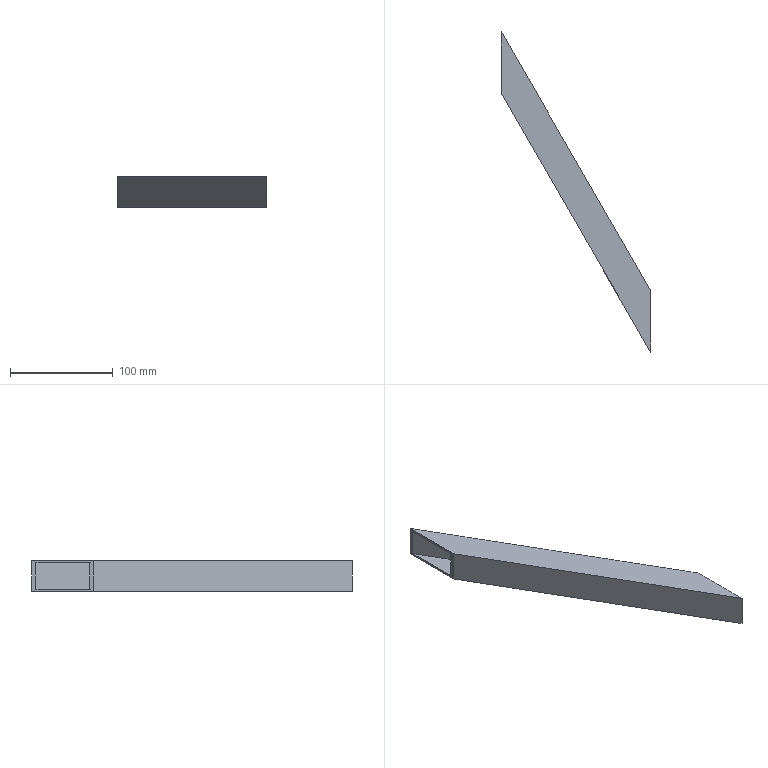Part | NX | features solid 2 | 1 solid | 10 faces | box 145 x 311.147 x 30 mm | volume 64960 mm3 | plane 10
STEP:
#1=CARTESIAN_POINT('',(-115.,495.,-45.));
#2=VERTEX_POINT('',#1);
#3=CARTESIAN_POINT('',(-115.,495.,-75.));
#4=VERTEX_POINT('',#3);
#5=CARTESIAN_POINT('',(-115.,495.,-75.));
#6=DIRECTION('',(0.,0.,-1.));
#7=VECTOR('',#6,1000.);
#8=LINE('',#5,#7);
#9=EDGE_CURVE('',#2,#4,#8,.T.);
#10=ORIENTED_EDGE('',*,*,#9,.F.);
#11=CARTESIAN_POINT('',(30.,243.853,-45.));
#12=VERTEX_POINT('',#11);
#13=CARTESIAN_POINT('',(-89.019,450.,-45.));
#14=DIRECTION('',(0.5,-0.866,0.));
#15=VECTOR('',#14,1000.);
#16=LINE('',#13,#15);
#17=EDGE_CURVE('',#2,#12,#16,.T.);
#18=ORIENTED_EDGE('',*,*,#17,.T.);
#19=CARTESIAN_POINT('',(30.,243.853,-75.));
#20=VERTEX_POINT('',#19);
#21=CARTESIAN_POINT('',(30.,243.853,-75.));
#22=DIRECTION('',(0.,0.,1.));
#23=VECTOR('',#22,1000.);
#24=LINE('',#21,#23);
#25=EDGE_CURVE('',#20,#12,#24,.T.);
#26=ORIENTED_EDGE('',*,*,#25,.F.);
#27=CARTESIAN_POINT('',(-89.019,450.,-75.));
#28=DIRECTION('',(0.5,-0.866,0.));
#29=VECTOR('',#28,1000.);
#30=LINE('',#27,#29);
#31=EDGE_CURVE('',#4,#20,#30,.T.);
#32=ORIENTED_EDGE('',*,*,#31,.F.);
#33=EDGE_LOOP('',(#10,#18,#26,#32));
#34=FACE_BOUND('',#33,.T.);
#35=CARTESIAN_POINT('',(-89.019,450.,-75.));
#36=DIRECTION('',(0.866,0.5,0.));
#37=DIRECTION('',(0.,0.,1.));
#38=AXIS2_PLACEMENT_3D('',#35,#36,#37);
#39=PLANE('',#38);
#40=ADVANCED_FACE('',(#34),#39,.T.);
#41=CARTESIAN_POINT('',(-115.,435.,-45.));
#42=VERTEX_POINT('',#41);
#43=CARTESIAN_POINT('',(30.,183.853,-45.));
#44=VERTEX_POINT('',#43);
#45=CARTESIAN_POINT('',(-115.,435.,-45.));
#46=DIRECTION('',(0.5,-0.866,0.));
#47=VECTOR('',#46,1000.);
#48=LINE('',#45,#47);
#49=EDGE_CURVE('',#42,#44,#48,.T.);
#50=ORIENTED_EDGE('',*,*,#49,.F.);
#51=CARTESIAN_POINT('',(-115.,435.,-75.));
#52=VERTEX_POINT('',#51);
#53=CARTESIAN_POINT('',(-115.,435.,-75.));
#54=DIRECTION('',(0.,0.,-1.));
#55=VECTOR('',#54,1000.);
#56=LINE('',#53,#55);
#57=EDGE_CURVE('',#42,#52,#56,.T.);
#58=ORIENTED_EDGE('',*,*,#57,.T.);
#59=CARTESIAN_POINT('',(30.,183.853,-75.));
#60=VERTEX_POINT('',#59);
#61=CARTESIAN_POINT('',(-115.,435.,-75.));
#62=DIRECTION('',(0.5,-0.866,0.));
#63=VECTOR('',#62,1000.);
#64=LINE('',#61,#63);
#65=EDGE_CURVE('',#52,#60,#64,.T.);
#66=ORIENTED_EDGE('',*,*,#65,.T.);
#67=CARTESIAN_POINT('',(30.,183.853,-75.));
#68=DIRECTION('',(0.,0.,1.));
#69=VECTOR('',#68,1000.);
#70=LINE('',#67,#69);
#71=EDGE_CURVE('',#60,#44,#70,.T.);
#72=ORIENTED_EDGE('',*,*,#71,.T.);
#73=EDGE_LOOP('',(#50,#58,#66,#72));
#74=FACE_BOUND('',#73,.T.);
#75=CARTESIAN_POINT('',(-115.,435.,-75.));
#76=DIRECTION('',(0.866,0.5,0.));
#77=DIRECTION('',(0.,0.,1.));
#78=AXIS2_PLACEMENT_3D('',#75,#76,#77);
#79=PLANE('',#78);
#80=ADVANCED_FACE('',(#74),#79,.F.);
#81=ORIENTED_EDGE('',*,*,#65,.F.);
#82=CARTESIAN_POINT('',(-115.,450.,-75.));
#83=DIRECTION('',(0.,1.,0.));
#84=VECTOR('',#83,1000.);
#85=LINE('',#82,#84);
#86=EDGE_CURVE('',#52,#4,#85,.T.);
#87=ORIENTED_EDGE('',*,*,#86,.T.);
#88=ORIENTED_EDGE('',*,*,#31,.T.);
#89=CARTESIAN_POINT('',(30.,450.,-75.));
#90=DIRECTION('',(0.,-1.,0.));
#91=VECTOR('',#90,1000.);
#92=LINE('',#89,#91);
#93=EDGE_CURVE('',#20,#60,#92,.T.);
#94=ORIENTED_EDGE('',*,*,#93,.T.);
#95=EDGE_LOOP('',(#81,#87,#88,#94));
#96=FACE_BOUND('',#95,.T.);
#97=CARTESIAN_POINT('',(-89.019,450.,-75.));
#98=DIRECTION('',(0.,0.,1.));
#99=DIRECTION('',(0.5,-0.866,0.));
#100=AXIS2_PLACEMENT_3D('',#97,#98,#99);
#101=PLANE('',#100);
#102=ADVANCED_FACE('',(#96),#101,.F.);
#103=ORIENTED_EDGE('',*,*,#17,.F.);
#104=CARTESIAN_POINT('',(-115.,450.,-45.));
#105=DIRECTION('',(0.,1.,0.));
#106=VECTOR('',#105,1000.);
#107=LINE('',#104,#106);
#108=EDGE_CURVE('',#2,#42,#107,.F.);
#109=ORIENTED_EDGE('',*,*,#108,.T.);
#110=ORIENTED_EDGE('',*,*,#49,.T.);
#111=CARTESIAN_POINT('',(30.,115.,-45.));
#112=DIRECTION('',(0.,1.,0.));
#113=VECTOR('',#112,1000.);
#114=LINE('',#111,#113);
#115=EDGE_CURVE('',#12,#44,#114,.F.);
#116=ORIENTED_EDGE('',*,*,#115,.F.);
#117=EDGE_LOOP('',(#103,#109,#110,#116));
#118=FACE_BOUND('',#117,.T.);
#119=CARTESIAN_POINT('',(-89.019,450.,-45.));
#120=DIRECTION('',(0.,0.,1.));
#121=DIRECTION('',(0.5,-0.866,0.));
#122=AXIS2_PLACEMENT_3D('',#119,#120,#121);
#123=PLANE('',#122);
#124=ADVANCED_FACE('',(#118),#123,.T.);
#125=ORIENTED_EDGE('',*,*,#115,.T.);
#126=ORIENTED_EDGE('',*,*,#71,.F.);
#127=ORIENTED_EDGE('',*,*,#93,.F.);
#128=ORIENTED_EDGE('',*,*,#25,.T.);
#129=EDGE_LOOP('',(#125,#126,#127,#128));
#130=FACE_BOUND('',#129,.T.);
#131=CARTESIAN_POINT('',(30.,239.853,-47.));
#132=VERTEX_POINT('',#131);
#133=CARTESIAN_POINT('',(30.,187.853,-47.));
#134=VERTEX_POINT('',#133);
#135=CARTESIAN_POINT('',(30.,115.,-47.));
#136=DIRECTION('',(0.,1.,0.));
#137=VECTOR('',#136,1000.);
#138=LINE('',#135,#137);
#139=EDGE_CURVE('',#132,#134,#138,.F.);
#140=ORIENTED_EDGE('',*,*,#139,.F.);
#141=CARTESIAN_POINT('',(30.,239.853,-73.));
#142=VERTEX_POINT('',#141);
#143=CARTESIAN_POINT('',(30.,239.853,-75.));
#144=DIRECTION('',(0.,0.,1.));
#145=VECTOR('',#144,1000.);
#146=LINE('',#143,#145);
#147=EDGE_CURVE('',#142,#132,#146,.T.);
#148=ORIENTED_EDGE('',*,*,#147,.F.);
#149=CARTESIAN_POINT('',(30.,187.853,-73.));
#150=VERTEX_POINT('',#149);
#151=CARTESIAN_POINT('',(30.,450.,-73.));
#152=DIRECTION('',(0.,-1.,0.));
#153=VECTOR('',#152,1000.);
#154=LINE('',#151,#153);
#155=EDGE_CURVE('',#142,#150,#154,.T.);
#156=ORIENTED_EDGE('',*,*,#155,.T.);
#157=CARTESIAN_POINT('',(30.,187.853,-75.));
#158=DIRECTION('',(0.,0.,1.));
#159=VECTOR('',#158,1000.);
#160=LINE('',#157,#159);
#161=EDGE_CURVE('',#150,#134,#160,.T.);
#162=ORIENTED_EDGE('',*,*,#161,.T.);
#163=EDGE_LOOP('',(#140,#148,#156,#162));
#164=FACE_BOUND('',#163,.T.);
#165=CARTESIAN_POINT('',(30.,115.,-45.));
#166=DIRECTION('',(-1.,0.,0.));
#167=DIRECTION('',(0.,-1.,0.));
#168=AXIS2_PLACEMENT_3D('',#165,#166,#167);
#169=PLANE('',#168);
#170=ADVANCED_FACE('',(#130,#164),#169,.F.);
#171=CARTESIAN_POINT('',(-115.,491.,-47.));
#172=VERTEX_POINT('',#171);
#173=CARTESIAN_POINT('',(-90.751,449.,-47.));
#174=DIRECTION('',(-0.5,0.866,0.));
#175=VECTOR('',#174,1000.);
#176=LINE('',#173,#175);
#177=EDGE_CURVE('',#172,#132,#176,.F.);
#178=ORIENTED_EDGE('',*,*,#177,.F.);
#179=CARTESIAN_POINT('',(-115.,491.,-73.));
#180=VERTEX_POINT('',#179);
#181=CARTESIAN_POINT('',(-115.,491.,-75.));
#182=DIRECTION('',(0.,0.,-1.));
#183=VECTOR('',#182,1000.);
#184=LINE('',#181,#183);
#185=EDGE_CURVE('',#172,#180,#184,.T.);
#186=ORIENTED_EDGE('',*,*,#185,.T.);
#187=CARTESIAN_POINT('',(-90.751,449.,-73.));
#188=DIRECTION('',(0.5,-0.866,0.));
#189=VECTOR('',#188,1000.);
#190=LINE('',#187,#189);
#191=EDGE_CURVE('',#180,#142,#190,.T.);
#192=ORIENTED_EDGE('',*,*,#191,.T.);
#193=ORIENTED_EDGE('',*,*,#147,.T.);
#194=EDGE_LOOP('',(#178,#186,#192,#193));
#195=FACE_BOUND('',#194,.T.);
#196=CARTESIAN_POINT('',(-90.751,449.,-75.));
#197=DIRECTION('',(0.866,0.5,0.));
#198=DIRECTION('',(0.,0.,1.));
#199=AXIS2_PLACEMENT_3D('',#196,#197,#198);
#200=PLANE('',#199);
#201=ADVANCED_FACE('',(#195),#200,.F.);
#202=CARTESIAN_POINT('',(-115.,439.,-47.));
#203=VERTEX_POINT('',#202);
#204=CARTESIAN_POINT('',(-115.,439.,-73.));
#205=VERTEX_POINT('',#204);
#206=CARTESIAN_POINT('',(-115.,439.,-75.));
#207=DIRECTION('',(0.,0.,-1.));
#208=VECTOR('',#207,1000.);
#209=LINE('',#206,#208);
#210=EDGE_CURVE('',#203,#205,#209,.T.);
#211=ORIENTED_EDGE('',*,*,#210,.F.);
#212=CARTESIAN_POINT('',(-113.268,436.,-47.));
#213=DIRECTION('',(-0.5,0.866,0.));
#214=VECTOR('',#213,1000.);
#215=LINE('',#212,#214);
#216=EDGE_CURVE('',#203,#134,#215,.F.);
#217=ORIENTED_EDGE('',*,*,#216,.T.);
#218=ORIENTED_EDGE('',*,*,#161,.F.);
#219=CARTESIAN_POINT('',(-113.268,436.,-73.));
#220=DIRECTION('',(0.5,-0.866,0.));
#221=VECTOR('',#220,1000.);
#222=LINE('',#219,#221);
#223=EDGE_CURVE('',#205,#150,#222,.T.);
#224=ORIENTED_EDGE('',*,*,#223,.F.);
#225=EDGE_LOOP('',(#211,#217,#218,#224));
#226=FACE_BOUND('',#225,.T.);
#227=CARTESIAN_POINT('',(-113.268,436.,-75.));
#228=DIRECTION('',(0.866,0.5,0.));
#229=DIRECTION('',(0.,0.,1.));
#230=AXIS2_PLACEMENT_3D('',#227,#228,#229);
#231=PLANE('',#230);
#232=ADVANCED_FACE('',(#226),#231,.T.);
#233=CARTESIAN_POINT('',(-115.,450.,-73.));
#234=DIRECTION('',(0.,1.,0.));
#235=VECTOR('',#234,1000.);
#236=LINE('',#233,#235);
#237=EDGE_CURVE('',#205,#180,#236,.T.);
#238=ORIENTED_EDGE('',*,*,#237,.F.);
#239=ORIENTED_EDGE('',*,*,#223,.T.);
#240=ORIENTED_EDGE('',*,*,#155,.F.);
#241=ORIENTED_EDGE('',*,*,#191,.F.);
#242=EDGE_LOOP('',(#238,#239,#240,#241));
#243=FACE_BOUND('',#242,.T.);
#244=CARTESIAN_POINT('',(-89.019,450.,-73.));
#245=DIRECTION('',(0.,0.,1.));
#246=DIRECTION('',(0.5,-0.866,0.));
#247=AXIS2_PLACEMENT_3D('',#244,#245,#246);
#248=PLANE('',#247);
#249=ADVANCED_FACE('',(#243),#248,.T.);
#250=CARTESIAN_POINT('',(-115.,450.,-47.));
#251=DIRECTION('',(0.,1.,0.));
#252=VECTOR('',#251,1000.);
#253=LINE('',#250,#252);
#254=EDGE_CURVE('',#172,#203,#253,.F.);
#255=ORIENTED_EDGE('',*,*,#254,.F.);
#256=ORIENTED_EDGE('',*,*,#177,.T.);
#257=ORIENTED_EDGE('',*,*,#139,.T.);
#258=ORIENTED_EDGE('',*,*,#216,.F.);
#259=EDGE_LOOP('',(#255,#256,#257,#258));
#260=FACE_BOUND('',#259,.T.);
#261=CARTESIAN_POINT('',(-89.019,450.,-47.));
#262=DIRECTION('',(0.,0.,1.));
#263=DIRECTION('',(0.5,-0.866,0.));
#264=AXIS2_PLACEMENT_3D('',#261,#262,#263);
#265=PLANE('',#264);
#266=ADVANCED_FACE('',(#260),#265,.F.);
#267=ORIENTED_EDGE('',*,*,#210,.T.);
#268=ORIENTED_EDGE('',*,*,#237,.T.);
#269=ORIENTED_EDGE('',*,*,#185,.F.);
#270=ORIENTED_EDGE('',*,*,#254,.T.);
#271=EDGE_LOOP('',(#267,#268,#269,#270));
#272=FACE_BOUND('',#271,.T.);
#273=ORIENTED_EDGE('',*,*,#108,.F.);
#274=ORIENTED_EDGE('',*,*,#9,.T.);
#275=ORIENTED_EDGE('',*,*,#86,.F.);
#276=ORIENTED_EDGE('',*,*,#57,.F.);
#277=EDGE_LOOP('',(#273,#274,#275,#276));
#278=FACE_BOUND('',#277,.T.);
#279=CARTESIAN_POINT('',(-115.,615.,-75.));
#280=DIRECTION('',(1.,0.,0.));
#281=DIRECTION('',(0.,0.,-1.));
#282=AXIS2_PLACEMENT_3D('',#279,#280,#281);
#283=PLANE('',#282);
#284=ADVANCED_FACE('',(#272,#278),#283,.F.);
#285=CLOSED_SHELL('',(#40,#80,#102,#124,#170,#201,#232,#249,#266,#284));
#286=MANIFOLD_SOLID_BREP('',#285);
#287=(LENGTH_UNIT()NAMED_UNIT(*)SI_UNIT(.MILLI.,.METRE.));
#288=UNCERTAINTY_MEASURE_WITH_UNIT(LENGTH_MEASURE(0.00001),#287,'','');
#289=(NAMED_UNIT(*)PLANE_ANGLE_UNIT()SI_UNIT($,.RADIAN.));
#290=(NAMED_UNIT(*)SI_UNIT($,.STERADIAN.)SOLID_ANGLE_UNIT());
#291=(GEOMETRIC_REPRESENTATION_CONTEXT(3)GLOBAL_UNCERTAINTY_ASSIGNED_CONTEXT((#288))GLOBAL_UNIT_ASSIGNED_CONTEXT((#287,#289,#290))REPRESENTATION_CONTEXT('',''));
#292=ADVANCED_BREP_SHAPE_REPRESENTATION('',(#286),#291);